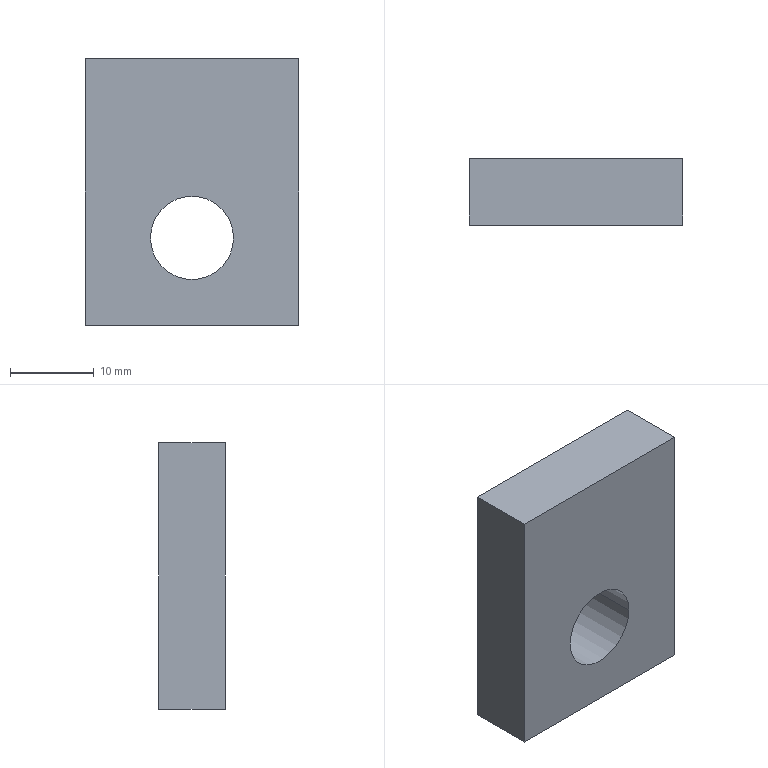Part | NX | features BREP 1 | 1 solid | 8 faces | box 25.4 x 7.938 x 31.75 mm | volume 5789 mm3 | plane 6 | cylinder 2 | commonest cylinder face diameters 9.906 x2
STEP:
#1=CARTESIAN_POINT('',(12.7,0.,-15.875));
#2=VERTEX_POINT('',#1);
#3=CARTESIAN_POINT('',(-12.7,0.,-15.875));
#4=VERTEX_POINT('',#3);
#5=CARTESIAN_POINT('',(12.7,0.,-15.875));
#6=DIRECTION('',(-1.,0.,0.));
#7=VECTOR('',#6,1000.);
#8=LINE('',#5,#7);
#9=EDGE_CURVE('',#2,#4,#8,.T.);
#10=ORIENTED_EDGE('',*,*,#9,.F.);
#11=CARTESIAN_POINT('',(12.7,0.,15.875));
#12=VERTEX_POINT('',#11);
#13=CARTESIAN_POINT('',(12.7,0.,15.875));
#14=DIRECTION('',(0.,0.,-1.));
#15=VECTOR('',#14,1000.);
#16=LINE('',#13,#15);
#17=EDGE_CURVE('',#12,#2,#16,.T.);
#18=ORIENTED_EDGE('',*,*,#17,.F.);
#19=CARTESIAN_POINT('',(-12.7,0.,15.875));
#20=VERTEX_POINT('',#19);
#21=CARTESIAN_POINT('',(-12.7,0.,15.875));
#22=DIRECTION('',(1.,0.,0.));
#23=VECTOR('',#22,1000.);
#24=LINE('',#21,#23);
#25=EDGE_CURVE('',#20,#12,#24,.T.);
#26=ORIENTED_EDGE('',*,*,#25,.F.);
#27=CARTESIAN_POINT('',(-12.7,0.,-15.875));
#28=DIRECTION('',(0.,0.,1.));
#29=VECTOR('',#28,1000.);
#30=LINE('',#27,#29);
#31=EDGE_CURVE('',#4,#20,#30,.T.);
#32=ORIENTED_EDGE('',*,*,#31,.F.);
#33=EDGE_LOOP('',(#10,#18,#26,#32));
#34=FACE_BOUND('',#33,.T.);
#35=CARTESIAN_POINT('',(-4.953,0.,-5.461));
#36=VERTEX_POINT('',#35);
#37=CARTESIAN_POINT('',(4.953,0.,-5.461));
#38=VERTEX_POINT('',#37);
#39=CARTESIAN_POINT('',(0.,0.,-5.461));
#40=DIRECTION('',(0.,-1.,0.));
#41=DIRECTION('',(-1.,0.,0.));
#42=AXIS2_PLACEMENT_3D('',#39,#40,#41);
#43=CIRCLE('',#42,4.953);
#44=EDGE_CURVE('',#36,#38,#43,.T.);
#45=ORIENTED_EDGE('',*,*,#44,.F.);
#46=CARTESIAN_POINT('',(0.,0.,-5.461));
#47=DIRECTION('',(0.,-1.,0.));
#48=DIRECTION('',(1.,0.,0.));
#49=AXIS2_PLACEMENT_3D('',#46,#47,#48);
#50=CIRCLE('',#49,4.953);
#51=EDGE_CURVE('',#38,#36,#50,.T.);
#52=ORIENTED_EDGE('',*,*,#51,.F.);
#53=EDGE_LOOP('',(#45,#52));
#54=FACE_BOUND('',#53,.T.);
#55=CARTESIAN_POINT('',(0.,0.,0.));
#56=DIRECTION('',(0.,1.,0.));
#57=DIRECTION('',(1.,0.,0.));
#58=AXIS2_PLACEMENT_3D('',#55,#56,#57);
#59=PLANE('',#58);
#60=ADVANCED_FACE('',(#34,#54),#59,.F.);
#61=CARTESIAN_POINT('',(-12.7,7.938,15.875));
#62=VERTEX_POINT('',#61);
#63=CARTESIAN_POINT('',(-12.7,0.,15.875));
#64=DIRECTION('',(0.,1.,0.));
#65=VECTOR('',#64,1000.);
#66=LINE('',#63,#65);
#67=EDGE_CURVE('',#20,#62,#66,.T.);
#68=ORIENTED_EDGE('',*,*,#67,.T.);
#69=CARTESIAN_POINT('',(-12.7,7.938,-15.875));
#70=VERTEX_POINT('',#69);
#71=CARTESIAN_POINT('',(-12.7,7.938,-15.875));
#72=DIRECTION('',(0.,0.,1.));
#73=VECTOR('',#72,1000.);
#74=LINE('',#71,#73);
#75=EDGE_CURVE('',#70,#62,#74,.T.);
#76=ORIENTED_EDGE('',*,*,#75,.F.);
#77=CARTESIAN_POINT('',(-12.7,0.,-15.875));
#78=DIRECTION('',(0.,1.,0.));
#79=VECTOR('',#78,1000.);
#80=LINE('',#77,#79);
#81=EDGE_CURVE('',#4,#70,#80,.T.);
#82=ORIENTED_EDGE('',*,*,#81,.F.);
#83=ORIENTED_EDGE('',*,*,#31,.T.);
#84=EDGE_LOOP('',(#68,#76,#82,#83));
#85=FACE_BOUND('',#84,.T.);
#86=CARTESIAN_POINT('',(-12.7,0.,-15.875));
#87=DIRECTION('',(-1.,0.,0.));
#88=DIRECTION('',(0.,0.,1.));
#89=AXIS2_PLACEMENT_3D('',#86,#87,#88);
#90=PLANE('',#89);
#91=ADVANCED_FACE('',(#85),#90,.T.);
#92=ORIENTED_EDGE('',*,*,#81,.T.);
#93=CARTESIAN_POINT('',(12.7,7.938,-15.875));
#94=VERTEX_POINT('',#93);
#95=CARTESIAN_POINT('',(12.7,7.938,-15.875));
#96=DIRECTION('',(-1.,0.,0.));
#97=VECTOR('',#96,1000.);
#98=LINE('',#95,#97);
#99=EDGE_CURVE('',#94,#70,#98,.T.);
#100=ORIENTED_EDGE('',*,*,#99,.F.);
#101=CARTESIAN_POINT('',(12.7,0.,-15.875));
#102=DIRECTION('',(0.,1.,0.));
#103=VECTOR('',#102,1000.);
#104=LINE('',#101,#103);
#105=EDGE_CURVE('',#2,#94,#104,.T.);
#106=ORIENTED_EDGE('',*,*,#105,.F.);
#107=ORIENTED_EDGE('',*,*,#9,.T.);
#108=EDGE_LOOP('',(#92,#100,#106,#107));
#109=FACE_BOUND('',#108,.T.);
#110=CARTESIAN_POINT('',(12.7,0.,-15.875));
#111=DIRECTION('',(0.,0.,-1.));
#112=DIRECTION('',(0.,-1.,0.));
#113=AXIS2_PLACEMENT_3D('',#110,#111,#112);
#114=PLANE('',#113);
#115=ADVANCED_FACE('',(#109),#114,.T.);
#116=ORIENTED_EDGE('',*,*,#105,.T.);
#117=CARTESIAN_POINT('',(12.7,7.938,15.875));
#118=VERTEX_POINT('',#117);
#119=CARTESIAN_POINT('',(12.7,7.938,15.875));
#120=DIRECTION('',(0.,0.,-1.));
#121=VECTOR('',#120,1000.);
#122=LINE('',#119,#121);
#123=EDGE_CURVE('',#118,#94,#122,.T.);
#124=ORIENTED_EDGE('',*,*,#123,.F.);
#125=CARTESIAN_POINT('',(12.7,0.,15.875));
#126=DIRECTION('',(0.,1.,0.));
#127=VECTOR('',#126,1000.);
#128=LINE('',#125,#127);
#129=EDGE_CURVE('',#12,#118,#128,.T.);
#130=ORIENTED_EDGE('',*,*,#129,.F.);
#131=ORIENTED_EDGE('',*,*,#17,.T.);
#132=EDGE_LOOP('',(#116,#124,#130,#131));
#133=FACE_BOUND('',#132,.T.);
#134=CARTESIAN_POINT('',(12.7,0.,15.875));
#135=DIRECTION('',(1.,0.,0.));
#136=DIRECTION('',(0.,1.,0.));
#137=AXIS2_PLACEMENT_3D('',#134,#135,#136);
#138=PLANE('',#137);
#139=ADVANCED_FACE('',(#133),#138,.T.);
#140=ORIENTED_EDGE('',*,*,#129,.T.);
#141=CARTESIAN_POINT('',(-12.7,7.938,15.875));
#142=DIRECTION('',(1.,0.,0.));
#143=VECTOR('',#142,1000.);
#144=LINE('',#141,#143);
#145=EDGE_CURVE('',#62,#118,#144,.T.);
#146=ORIENTED_EDGE('',*,*,#145,.F.);
#147=ORIENTED_EDGE('',*,*,#67,.F.);
#148=ORIENTED_EDGE('',*,*,#25,.T.);
#149=EDGE_LOOP('',(#140,#146,#147,#148));
#150=FACE_BOUND('',#149,.T.);
#151=CARTESIAN_POINT('',(-12.7,0.,15.875));
#152=DIRECTION('',(0.,0.,1.));
#153=DIRECTION('',(1.,0.,0.));
#154=AXIS2_PLACEMENT_3D('',#151,#152,#153);
#155=PLANE('',#154);
#156=ADVANCED_FACE('',(#150),#155,.T.);
#157=ORIENTED_EDGE('',*,*,#145,.T.);
#158=ORIENTED_EDGE('',*,*,#123,.T.);
#159=ORIENTED_EDGE('',*,*,#99,.T.);
#160=ORIENTED_EDGE('',*,*,#75,.T.);
#161=EDGE_LOOP('',(#157,#158,#159,#160));
#162=FACE_BOUND('',#161,.T.);
#163=CARTESIAN_POINT('',(-4.953,7.938,-5.461));
#164=VERTEX_POINT('',#163);
#165=CARTESIAN_POINT('',(4.953,7.938,-5.461));
#166=VERTEX_POINT('',#165);
#167=CARTESIAN_POINT('',(0.,7.938,-5.461));
#168=DIRECTION('',(0.,-1.,0.));
#169=DIRECTION('',(-1.,0.,0.));
#170=AXIS2_PLACEMENT_3D('',#167,#168,#169);
#171=CIRCLE('',#170,4.953);
#172=EDGE_CURVE('',#164,#166,#171,.T.);
#173=ORIENTED_EDGE('',*,*,#172,.T.);
#174=CARTESIAN_POINT('',(0.,7.938,-5.461));
#175=DIRECTION('',(0.,-1.,0.));
#176=DIRECTION('',(1.,0.,0.));
#177=AXIS2_PLACEMENT_3D('',#174,#175,#176);
#178=CIRCLE('',#177,4.953);
#179=EDGE_CURVE('',#166,#164,#178,.T.);
#180=ORIENTED_EDGE('',*,*,#179,.T.);
#181=EDGE_LOOP('',(#173,#180));
#182=FACE_BOUND('',#181,.T.);
#183=CARTESIAN_POINT('',(0.,7.938,0.));
#184=DIRECTION('',(0.,1.,0.));
#185=DIRECTION('',(1.,0.,0.));
#186=AXIS2_PLACEMENT_3D('',#183,#184,#185);
#187=PLANE('',#186);
#188=ADVANCED_FACE('',(#162,#182),#187,.T.);
#189=CARTESIAN_POINT('',(-4.953,7.938,-5.461));
#190=DIRECTION('',(0.,-1.,0.));
#191=VECTOR('',#190,1000.);
#192=LINE('',#189,#191);
#193=EDGE_CURVE('',#164,#36,#192,.T.);
#194=ORIENTED_EDGE('',*,*,#193,.F.);
#195=ORIENTED_EDGE('',*,*,#179,.F.);
#196=CARTESIAN_POINT('',(4.953,7.938,-5.461));
#197=DIRECTION('',(0.,-1.,0.));
#198=VECTOR('',#197,1000.);
#199=LINE('',#196,#198);
#200=EDGE_CURVE('',#166,#38,#199,.T.);
#201=ORIENTED_EDGE('',*,*,#200,.T.);
#202=ORIENTED_EDGE('',*,*,#51,.T.);
#203=EDGE_LOOP('',(#194,#195,#201,#202));
#204=FACE_BOUND('',#203,.T.);
#205=CARTESIAN_POINT('',(0.,7.938,-5.461));
#206=DIRECTION('',(0.,-1.,0.));
#207=DIRECTION('',(1.,0.,0.));
#208=AXIS2_PLACEMENT_3D('',#205,#206,#207);
#209=CYLINDRICAL_SURFACE('',#208,4.953);
#210=ADVANCED_FACE('',(#204),#209,.F.);
#211=ORIENTED_EDGE('',*,*,#200,.F.);
#212=ORIENTED_EDGE('',*,*,#172,.F.);
#213=ORIENTED_EDGE('',*,*,#193,.T.);
#214=ORIENTED_EDGE('',*,*,#44,.T.);
#215=EDGE_LOOP('',(#211,#212,#213,#214));
#216=FACE_BOUND('',#215,.T.);
#217=CARTESIAN_POINT('',(0.,7.938,-5.461));
#218=DIRECTION('',(0.,-1.,0.));
#219=DIRECTION('',(1.,0.,0.));
#220=AXIS2_PLACEMENT_3D('',#217,#218,#219);
#221=CYLINDRICAL_SURFACE('',#220,4.953);
#222=ADVANCED_FACE('',(#216),#221,.F.);
#223=CLOSED_SHELL('',(#60,#91,#115,#139,#156,#188,#210,#222));
#224=MANIFOLD_SOLID_BREP('',#223);
#225=(LENGTH_UNIT()NAMED_UNIT(*)SI_UNIT(.MILLI.,.METRE.));
#226=UNCERTAINTY_MEASURE_WITH_UNIT(LENGTH_MEASURE(0.00001),#225,'','');
#227=(NAMED_UNIT(*)PLANE_ANGLE_UNIT()SI_UNIT($,.RADIAN.));
#228=(NAMED_UNIT(*)SI_UNIT($,.STERADIAN.)SOLID_ANGLE_UNIT());
#229=(GEOMETRIC_REPRESENTATION_CONTEXT(3)GLOBAL_UNCERTAINTY_ASSIGNED_CONTEXT((#226))GLOBAL_UNIT_ASSIGNED_CONTEXT((#225,#227,#228))REPRESENTATION_CONTEXT('',''));
#230=ADVANCED_BREP_SHAPE_REPRESENTATION('',(#224),#229);